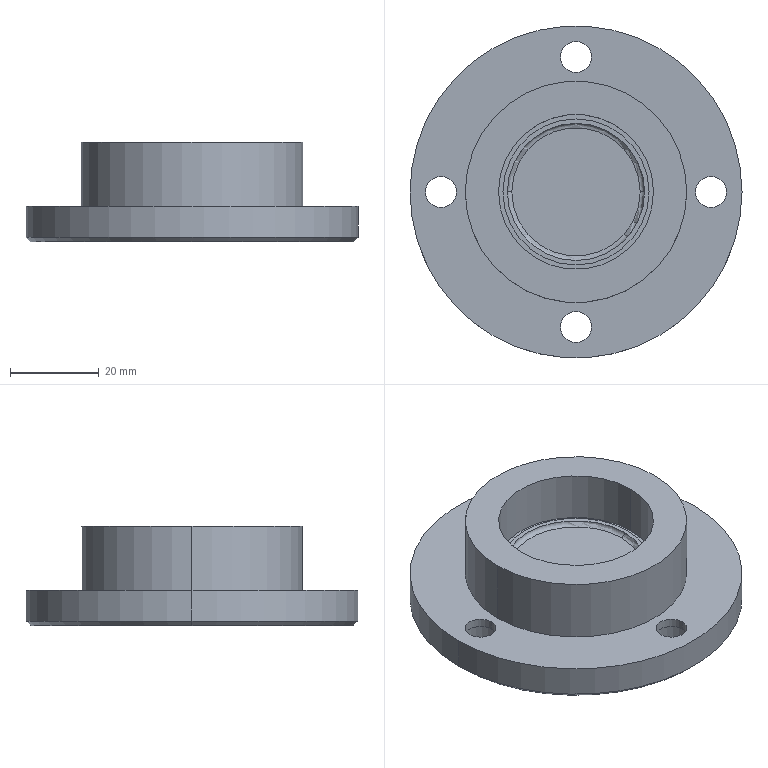Part | SolidWorks | features ICE 7, Chamfer 1, CirPattern 1, Extrusion 1, Fillet 1 | 1 solid | 41 faces | box 75 x 75 x 22.5 mm | volume 47960 mm3 | cylinder 24 | plane 11 | torus 4 | cone 2 | commonest cylinder face diameters 7 x8 11 x8 33 x2 35 x2 50 x2 75 x2
STEP:
#1=CARTESIAN_POINT('',(-36.5,0.,0.));
#2=VERTEX_POINT('',#1);
#3=CARTESIAN_POINT('',(36.5,0.,0.));
#4=VERTEX_POINT('',#3);
#5=CARTESIAN_POINT('',(0.,0.,0.));
#6=DIRECTION('',(0.,0.,-1.));
#7=DIRECTION('',(1.,0.,0.));
#8=AXIS2_PLACEMENT_3D('',#5,#6,#7);
#9=CIRCLE('',#8,36.5);
#10=EDGE_CURVE('',#2,#4,#9,.T.);
#11=ORIENTED_EDGE('',*,*,#10,.F.);
#12=CARTESIAN_POINT('',(-37.5,0.,1.));
#13=VERTEX_POINT('',#12);
#14=CARTESIAN_POINT('',(-37.5,0.,1.));
#15=DIRECTION('',(-0.7071,0.,0.7071));
#16=VECTOR('',#15,1000.);
#17=LINE('',#14,#16);
#18=EDGE_CURVE('',#2,#13,#17,.T.);
#19=ORIENTED_EDGE('',*,*,#18,.T.);
#20=CARTESIAN_POINT('',(37.5,0.,1.));
#21=VERTEX_POINT('',#20);
#22=CARTESIAN_POINT('',(0.,0.,1.));
#23=DIRECTION('',(0.,0.,1.));
#24=DIRECTION('',(1.,0.,0.));
#25=AXIS2_PLACEMENT_3D('',#22,#23,#24);
#26=CIRCLE('',#25,37.5);
#27=EDGE_CURVE('',#21,#13,#26,.T.);
#28=ORIENTED_EDGE('',*,*,#27,.F.);
#29=CARTESIAN_POINT('',(37.5,0.,1.));
#30=DIRECTION('',(0.7071,0.,0.7071));
#31=VECTOR('',#30,1000.);
#32=LINE('',#29,#31);
#33=EDGE_CURVE('',#4,#21,#32,.T.);
#34=ORIENTED_EDGE('',*,*,#33,.F.);
#35=EDGE_LOOP('',(#11,#19,#28,#34));
#36=FACE_OUTER_BOUND('',#35,.T.);
#37=CARTESIAN_POINT('',(0.,0.,1.));
#38=DIRECTION('',(0.,0.,1.));
#39=DIRECTION('',(1.,0.,0.));
#40=AXIS2_PLACEMENT_3D('',#37,#38,#39);
#41=CONICAL_SURFACE('',#40,37.5,0.7854);
#42=ADVANCED_FACE('',(#36),#41,.T.);
#43=CARTESIAN_POINT('',(-14.5,0.,10.5));
#44=VERTEX_POINT('',#43);
#45=CARTESIAN_POINT('',(14.5,0.,10.5));
#46=VERTEX_POINT('',#45);
#47=CARTESIAN_POINT('',(0.,0.,10.5));
#48=DIRECTION('',(0.,0.,1.));
#49=DIRECTION('',(1.,0.,0.));
#50=AXIS2_PLACEMENT_3D('',#47,#48,#49);
#51=CIRCLE('',#50,14.5);
#52=EDGE_CURVE('',#44,#46,#51,.T.);
#53=ORIENTED_EDGE('',*,*,#52,.F.);
#54=CARTESIAN_POINT('',(-15.5,0.,11.5));
#55=VERTEX_POINT('',#54);
#56=CARTESIAN_POINT('',(-14.5,0.,11.5));
#57=DIRECTION('',(0.,1.,0.));
#58=DIRECTION('',(-1.,0.,0.));
#59=AXIS2_PLACEMENT_3D('',#56,#57,#58);
#60=CIRCLE('',#59,1.);
#61=EDGE_CURVE('',#44,#55,#60,.T.);
#62=ORIENTED_EDGE('',*,*,#61,.T.);
#63=CARTESIAN_POINT('',(15.5,0.,11.5));
#64=VERTEX_POINT('',#63);
#65=CARTESIAN_POINT('',(0.,0.,11.5));
#66=DIRECTION('',(0.,0.,1.));
#67=DIRECTION('',(1.,0.,0.));
#68=AXIS2_PLACEMENT_3D('',#65,#66,#67);
#69=CIRCLE('',#68,15.5);
#70=EDGE_CURVE('',#55,#64,#69,.T.);
#71=ORIENTED_EDGE('',*,*,#70,.T.);
#72=CARTESIAN_POINT('',(14.5,0.,11.5));
#73=DIRECTION('',(0.,-1.,0.));
#74=DIRECTION('',(0.,0.,-1.));
#75=AXIS2_PLACEMENT_3D('',#72,#73,#74);
#76=CIRCLE('',#75,1.);
#77=EDGE_CURVE('',#46,#64,#76,.T.);
#78=ORIENTED_EDGE('',*,*,#77,.F.);
#79=EDGE_LOOP('',(#53,#62,#71,#78));
#80=FACE_OUTER_BOUND('',#79,.T.);
#81=CARTESIAN_POINT('',(0.,0.,11.5));
#82=DIRECTION('',(0.,0.,1.));
#83=DIRECTION('',(1.,0.,0.));
#84=AXIS2_PLACEMENT_3D('',#81,#82,#83);
#85=TOROIDAL_SURFACE('',#84,14.5,1.);
#86=ADVANCED_FACE('',(#80),#85,.F.);
#87=CARTESIAN_POINT('',(23.,0.,1.));
#88=VERTEX_POINT('',#87);
#89=CARTESIAN_POINT('',(-23.,0.,1.));
#90=VERTEX_POINT('',#89);
#91=CARTESIAN_POINT('',(0.,0.,1.));
#92=DIRECTION('',(0.,0.,-1.));
#93=DIRECTION('',(-1.,0.,0.));
#94=AXIS2_PLACEMENT_3D('',#91,#92,#93);
#95=CIRCLE('',#94,23.);
#96=EDGE_CURVE('',#88,#90,#95,.T.);
#97=ORIENTED_EDGE('',*,*,#96,.F.);
#98=CARTESIAN_POINT('',(24.,0.,0.));
#99=VERTEX_POINT('',#98);
#100=CARTESIAN_POINT('',(23.,0.,0.));
#101=DIRECTION('',(0.,1.,0.));
#102=DIRECTION('',(-1.,0.,0.));
#103=AXIS2_PLACEMENT_3D('',#100,#101,#102);
#104=CIRCLE('',#103,1.);
#105=EDGE_CURVE('',#88,#99,#104,.T.);
#106=ORIENTED_EDGE('',*,*,#105,.T.);
#107=CARTESIAN_POINT('',(-24.,0.,0.));
#108=VERTEX_POINT('',#107);
#109=CARTESIAN_POINT('',(0.,0.,0.));
#110=DIRECTION('',(0.,0.,-1.));
#111=DIRECTION('',(-1.,0.,0.));
#112=AXIS2_PLACEMENT_3D('',#109,#110,#111);
#113=CIRCLE('',#112,24.);
#114=EDGE_CURVE('',#99,#108,#113,.T.);
#115=ORIENTED_EDGE('',*,*,#114,.T.);
#116=CARTESIAN_POINT('',(-23.,0.,0.));
#117=DIRECTION('',(0.,-1.,0.));
#118=DIRECTION('',(0.,0.,-1.));
#119=AXIS2_PLACEMENT_3D('',#116,#117,#118);
#120=CIRCLE('',#119,1.);
#121=EDGE_CURVE('',#90,#108,#120,.T.);
#122=ORIENTED_EDGE('',*,*,#121,.F.);
#123=EDGE_LOOP('',(#97,#106,#115,#122));
#124=FACE_OUTER_BOUND('',#123,.T.);
#125=CARTESIAN_POINT('',(0.,0.,0.));
#126=DIRECTION('',(0.,0.,-1.));
#127=DIRECTION('',(-1.,0.,0.));
#128=AXIS2_PLACEMENT_3D('',#125,#126,#127);
#129=TOROIDAL_SURFACE('',#128,23.,1.);
#130=ADVANCED_FACE('',(#124),#129,.F.);
#131=CARTESIAN_POINT('',(16.5,0.,11.));
#132=VERTEX_POINT('',#131);
#133=CARTESIAN_POINT('',(-16.5,0.,11.));
#134=VERTEX_POINT('',#133);
#135=CARTESIAN_POINT('',(0.,0.,11.));
#136=DIRECTION('',(0.,0.,1.));
#137=DIRECTION('',(1.,0.,0.));
#138=AXIS2_PLACEMENT_3D('',#135,#136,#137);
#139=CIRCLE('',#138,16.5);
#140=EDGE_CURVE('',#132,#134,#139,.T.);
#141=ORIENTED_EDGE('',*,*,#140,.T.);
#142=CARTESIAN_POINT('',(-16.5,0.,11.5));
#143=VERTEX_POINT('',#142);
#144=CARTESIAN_POINT('',(-16.5,0.,11.));
#145=DIRECTION('',(0.,0.,1.));
#146=VECTOR('',#145,1000.);
#147=LINE('',#144,#146);
#148=EDGE_CURVE('',#134,#143,#147,.T.);
#149=ORIENTED_EDGE('',*,*,#148,.T.);
#150=CARTESIAN_POINT('',(16.5,0.,11.5));
#151=VERTEX_POINT('',#150);
#152=CARTESIAN_POINT('',(0.,0.,11.5));
#153=DIRECTION('',(0.,0.,1.));
#154=DIRECTION('',(1.,0.,0.));
#155=AXIS2_PLACEMENT_3D('',#152,#153,#154);
#156=CIRCLE('',#155,16.5);
#157=EDGE_CURVE('',#151,#143,#156,.T.);
#158=ORIENTED_EDGE('',*,*,#157,.F.);
#159=CARTESIAN_POINT('',(16.5,0.,11.));
#160=DIRECTION('',(0.,0.,1.));
#161=VECTOR('',#160,1000.);
#162=LINE('',#159,#161);
#163=EDGE_CURVE('',#132,#151,#162,.T.);
#164=ORIENTED_EDGE('',*,*,#163,.F.);
#165=EDGE_LOOP('',(#141,#149,#158,#164));
#166=FACE_OUTER_BOUND('',#165,.T.);
#167=CARTESIAN_POINT('',(0.,0.,11.));
#168=DIRECTION('',(0.,0.,1.));
#169=DIRECTION('',(1.,0.,0.));
#170=AXIS2_PLACEMENT_3D('',#167,#168,#169);
#171=CYLINDRICAL_SURFACE('',#170,16.5);
#172=ADVANCED_FACE('',(#166),#171,.T.);
#173=CARTESIAN_POINT('',(-17.5,0.,11.));
#174=VERTEX_POINT('',#173);
#175=CARTESIAN_POINT('',(17.5,0.,11.));
#176=VERTEX_POINT('',#175);
#177=CARTESIAN_POINT('',(0.,0.,11.));
#178=DIRECTION('',(0.,0.,1.));
#179=DIRECTION('',(1.,0.,0.));
#180=AXIS2_PLACEMENT_3D('',#177,#178,#179);
#181=CIRCLE('',#180,17.5);
#182=EDGE_CURVE('',#174,#176,#181,.T.);
#183=ORIENTED_EDGE('',*,*,#182,.F.);
#184=CARTESIAN_POINT('',(-17.5,0.,22.5));
#185=VERTEX_POINT('',#184);
#186=CARTESIAN_POINT('',(-17.5,0.,11.5));
#187=DIRECTION('',(0.,0.,1.));
#188=VECTOR('',#187,1000.);
#189=LINE('',#186,#188);
#190=EDGE_CURVE('',#174,#185,#189,.T.);
#191=ORIENTED_EDGE('',*,*,#190,.T.);
#192=CARTESIAN_POINT('',(17.5,0.,22.5));
#193=VERTEX_POINT('',#192);
#194=CARTESIAN_POINT('',(0.,0.,22.5));
#195=DIRECTION('',(0.,0.,1.));
#196=DIRECTION('',(1.,0.,0.));
#197=AXIS2_PLACEMENT_3D('',#194,#195,#196);
#198=CIRCLE('',#197,17.5);
#199=EDGE_CURVE('',#185,#193,#198,.T.);
#200=ORIENTED_EDGE('',*,*,#199,.T.);
#201=CARTESIAN_POINT('',(17.5,0.,11.5));
#202=DIRECTION('',(0.,0.,1.));
#203=VECTOR('',#202,1000.);
#204=LINE('',#201,#203);
#205=EDGE_CURVE('',#176,#193,#204,.T.);
#206=ORIENTED_EDGE('',*,*,#205,.F.);
#207=EDGE_LOOP('',(#183,#191,#200,#206));
#208=FACE_OUTER_BOUND('',#207,.T.);
#209=CARTESIAN_POINT('',(0.,0.,11.5));
#210=DIRECTION('',(0.,0.,1.));
#211=DIRECTION('',(1.,0.,0.));
#212=AXIS2_PLACEMENT_3D('',#209,#210,#211);
#213=CYLINDRICAL_SURFACE('',#212,17.5);
#214=ADVANCED_FACE('',(#208),#213,.F.);
#215=CARTESIAN_POINT('',(27.,0.,8.));
#216=VERTEX_POINT('',#215);
#217=CARTESIAN_POINT('',(34.,0.,8.));
#218=VERTEX_POINT('',#217);
#219=CARTESIAN_POINT('',(30.5,0.,8.));
#220=DIRECTION('',(0.,0.,1.));
#221=DIRECTION('',(1.,0.,0.));
#222=AXIS2_PLACEMENT_3D('',#219,#220,#221);
#223=CIRCLE('',#222,3.5);
#224=EDGE_CURVE('',#216,#218,#223,.T.);
#225=ORIENTED_EDGE('',*,*,#224,.T.);
#226=CARTESIAN_POINT('',(34.,0.,6.));
#227=VERTEX_POINT('',#226);
#228=CARTESIAN_POINT('',(34.,0.,27.));
#229=DIRECTION('',(0.,0.,-1.));
#230=VECTOR('',#229,1000.);
#231=LINE('',#228,#230);
#232=EDGE_CURVE('',#218,#227,#231,.T.);
#233=ORIENTED_EDGE('',*,*,#232,.T.);
#234=CARTESIAN_POINT('',(27.,0.,6.));
#235=VERTEX_POINT('',#234);
#236=CARTESIAN_POINT('',(30.5,0.,6.));
#237=DIRECTION('',(0.,0.,-1.));
#238=DIRECTION('',(0.,1.,0.));
#239=AXIS2_PLACEMENT_3D('',#236,#237,#238);
#240=CIRCLE('',#239,3.5);
#241=EDGE_CURVE('',#227,#235,#240,.T.);
#242=ORIENTED_EDGE('',*,*,#241,.T.);
#243=CARTESIAN_POINT('',(27.,0.,27.));
#244=DIRECTION('',(0.,0.,-1.));
#245=VECTOR('',#244,1000.);
#246=LINE('',#243,#245);
#247=EDGE_CURVE('',#216,#235,#246,.T.);
#248=ORIENTED_EDGE('',*,*,#247,.F.);
#249=EDGE_LOOP('',(#225,#233,#242,#248));
#250=FACE_OUTER_BOUND('',#249,.T.);
#251=CARTESIAN_POINT('',(30.5,0.,27.));
#252=DIRECTION('',(0.,0.,-1.));
#253=DIRECTION('',(-1.,0.,0.));
#254=AXIS2_PLACEMENT_3D('',#251,#252,#253);
#255=CYLINDRICAL_SURFACE('',#254,3.5);
#256=ADVANCED_FACE('',(#250),#255,.F.);
#257=CARTESIAN_POINT('',(-3.5,-30.5,8.));
#258=VERTEX_POINT('',#257);
#259=CARTESIAN_POINT('',(3.5,-30.5,8.));
#260=VERTEX_POINT('',#259);
#261=CARTESIAN_POINT('',(0.,-30.5,8.));
#262=DIRECTION('',(0.,0.,1.));
#263=DIRECTION('',(1.,0.,0.));
#264=AXIS2_PLACEMENT_3D('',#261,#262,#263);
#265=CIRCLE('',#264,3.5);
#266=EDGE_CURVE('',#258,#260,#265,.T.);
#267=ORIENTED_EDGE('',*,*,#266,.T.);
#268=CARTESIAN_POINT('',(3.5,-30.5,6.));
#269=VERTEX_POINT('',#268);
#270=CARTESIAN_POINT('',(3.5,-30.5,27.));
#271=DIRECTION('',(0.,0.,-1.));
#272=VECTOR('',#271,1000.);
#273=LINE('',#270,#272);
#274=EDGE_CURVE('',#260,#269,#273,.T.);
#275=ORIENTED_EDGE('',*,*,#274,.T.);
#276=CARTESIAN_POINT('',(-3.5,-30.5,6.));
#277=VERTEX_POINT('',#276);
#278=CARTESIAN_POINT('',(0.,-30.5,6.));
#279=DIRECTION('',(0.,0.,-1.));
#280=DIRECTION('',(1.,0.,0.));
#281=AXIS2_PLACEMENT_3D('',#278,#279,#280);
#282=CIRCLE('',#281,3.5);
#283=EDGE_CURVE('',#269,#277,#282,.T.);
#284=ORIENTED_EDGE('',*,*,#283,.T.);
#285=CARTESIAN_POINT('',(-3.5,-30.5,27.));
#286=DIRECTION('',(0.,0.,-1.));
#287=VECTOR('',#286,1000.);
#288=LINE('',#285,#287);
#289=EDGE_CURVE('',#258,#277,#288,.T.);
#290=ORIENTED_EDGE('',*,*,#289,.F.);
#291=EDGE_LOOP('',(#267,#275,#284,#290));
#292=FACE_OUTER_BOUND('',#291,.T.);
#293=CARTESIAN_POINT('',(0.,-30.5,27.));
#294=DIRECTION('',(0.,0.,-1.));
#295=DIRECTION('',(-1.,0.,0.));
#296=AXIS2_PLACEMENT_3D('',#293,#294,#295);
#297=CYLINDRICAL_SURFACE('',#296,3.5);
#298=ADVANCED_FACE('',(#292),#297,.F.);
#299=CARTESIAN_POINT('',(-34.,0.,8.));
#300=VERTEX_POINT('',#299);
#301=CARTESIAN_POINT('',(-27.,0.,8.));
#302=VERTEX_POINT('',#301);
#303=CARTESIAN_POINT('',(-30.5,0.,8.));
#304=DIRECTION('',(0.,0.,1.));
#305=DIRECTION('',(1.,0.,0.));
#306=AXIS2_PLACEMENT_3D('',#303,#304,#305);
#307=CIRCLE('',#306,3.5);
#308=EDGE_CURVE('',#300,#302,#307,.T.);
#309=ORIENTED_EDGE('',*,*,#308,.T.);
#310=CARTESIAN_POINT('',(-27.,0.,6.));
#311=VERTEX_POINT('',#310);
#312=CARTESIAN_POINT('',(-27.,0.,27.));
#313=DIRECTION('',(0.,0.,-1.));
#314=VECTOR('',#313,1000.);
#315=LINE('',#312,#314);
#316=EDGE_CURVE('',#302,#311,#315,.T.);
#317=ORIENTED_EDGE('',*,*,#316,.T.);
#318=CARTESIAN_POINT('',(-34.,0.,6.));
#319=VERTEX_POINT('',#318);
#320=CARTESIAN_POINT('',(-30.5,0.,6.));
#321=DIRECTION('',(0.,0.,-1.));
#322=DIRECTION('',(0.,-1.,0.));
#323=AXIS2_PLACEMENT_3D('',#320,#321,#322);
#324=CIRCLE('',#323,3.5);
#325=EDGE_CURVE('',#311,#319,#324,.T.);
#326=ORIENTED_EDGE('',*,*,#325,.T.);
#327=CARTESIAN_POINT('',(-34.,0.,27.));
#328=DIRECTION('',(0.,0.,-1.));
#329=VECTOR('',#328,1000.);
#330=LINE('',#327,#329);
#331=EDGE_CURVE('',#300,#319,#330,.T.);
#332=ORIENTED_EDGE('',*,*,#331,.F.);
#333=EDGE_LOOP('',(#309,#317,#326,#332));
#334=FACE_OUTER_BOUND('',#333,.T.);
#335=CARTESIAN_POINT('',(-30.5,0.,27.));
#336=DIRECTION('',(0.,0.,-1.));
#337=DIRECTION('',(-1.,0.,0.));
#338=AXIS2_PLACEMENT_3D('',#335,#336,#337);
#339=CYLINDRICAL_SURFACE('',#338,3.5);
#340=ADVANCED_FACE('',(#334),#339,.F.);
#341=CARTESIAN_POINT('',(36.,0.,6.));
#342=VERTEX_POINT('',#341);
#343=CARTESIAN_POINT('',(25.,0.,6.));
#344=VERTEX_POINT('',#343);
#345=CARTESIAN_POINT('',(30.5,0.,6.));
#346=DIRECTION('',(0.,0.,-1.));
#347=DIRECTION('',(0.,1.,0.));
#348=AXIS2_PLACEMENT_3D('',#345,#346,#347);
#349=CIRCLE('',#348,5.5);
#350=EDGE_CURVE('',#342,#344,#349,.T.);
#351=ORIENTED_EDGE('',*,*,#350,.F.);
#352=CARTESIAN_POINT('',(36.,0.,0.));
#353=VERTEX_POINT('',#352);
#354=CARTESIAN_POINT('',(36.,0.,6.));
#355=DIRECTION('',(0.,0.,-1.));
#356=VECTOR('',#355,1000.);
#357=LINE('',#354,#356);
#358=EDGE_CURVE('',#342,#353,#357,.T.);
#359=ORIENTED_EDGE('',*,*,#358,.T.);
#360=CARTESIAN_POINT('',(25.,0.,0.));
#361=VERTEX_POINT('',#360);
#362=CARTESIAN_POINT('',(30.5,0.,0.));
#363=DIRECTION('',(0.,0.,-1.));
#364=DIRECTION('',(0.,1.,0.));
#365=AXIS2_PLACEMENT_3D('',#362,#363,#364);
#366=CIRCLE('',#365,5.5);
#367=EDGE_CURVE('',#353,#361,#366,.T.);
#368=ORIENTED_EDGE('',*,*,#367,.T.);
#369=CARTESIAN_POINT('',(25.,0.,6.));
#370=DIRECTION('',(0.,0.,-1.));
#371=VECTOR('',#370,1000.);
#372=LINE('',#369,#371);
#373=EDGE_CURVE('',#344,#361,#372,.T.);
#374=ORIENTED_EDGE('',*,*,#373,.F.);
#375=EDGE_LOOP('',(#351,#359,#368,#374));
#376=FACE_OUTER_BOUND('',#375,.T.);
#377=CARTESIAN_POINT('',(30.5,0.,6.));
#378=DIRECTION('',(0.,0.,-1.));
#379=DIRECTION('',(-1.,0.,0.));
#380=AXIS2_PLACEMENT_3D('',#377,#378,#379);
#381=CYLINDRICAL_SURFACE('',#380,5.5);
#382=ADVANCED_FACE('',(#376),#381,.F.);
#383=CARTESIAN_POINT('',(5.5,-30.5,6.));
#384=VERTEX_POINT('',#383);
#385=CARTESIAN_POINT('',(-5.5,-30.5,6.));
#386=VERTEX_POINT('',#385);
#387=CARTESIAN_POINT('',(0.,-30.5,6.));
#388=DIRECTION('',(0.,0.,-1.));
#389=DIRECTION('',(1.,0.,0.));
#390=AXIS2_PLACEMENT_3D('',#387,#388,#389);
#391=CIRCLE('',#390,5.5);
#392=EDGE_CURVE('',#384,#386,#391,.T.);
#393=ORIENTED_EDGE('',*,*,#392,.F.);
#394=CARTESIAN_POINT('',(5.5,-30.5,0.));
#395=VERTEX_POINT('',#394);
#396=CARTESIAN_POINT('',(5.5,-30.5,6.));
#397=DIRECTION('',(0.,0.,-1.));
#398=VECTOR('',#397,1000.);
#399=LINE('',#396,#398);
#400=EDGE_CURVE('',#384,#395,#399,.T.);
#401=ORIENTED_EDGE('',*,*,#400,.T.);
#402=CARTESIAN_POINT('',(-5.5,-30.5,0.));
#403=VERTEX_POINT('',#402);
#404=CARTESIAN_POINT('',(0.,-30.5,0.));
#405=DIRECTION('',(0.,0.,-1.));
#406=DIRECTION('',(1.,0.,0.));
#407=AXIS2_PLACEMENT_3D('',#404,#405,#406);
#408=CIRCLE('',#407,5.5);
#409=EDGE_CURVE('',#395,#403,#408,.T.);
#410=ORIENTED_EDGE('',*,*,#409,.T.);
#411=CARTESIAN_POINT('',(-5.5,-30.5,6.));
#412=DIRECTION('',(0.,0.,-1.));
#413=VECTOR('',#412,1000.);
#414=LINE('',#411,#413);
#415=EDGE_CURVE('',#386,#403,#414,.T.);
#416=ORIENTED_EDGE('',*,*,#415,.F.);
#417=EDGE_LOOP('',(#393,#401,#410,#416));
#418=FACE_OUTER_BOUND('',#417,.T.);
#419=CARTESIAN_POINT('',(0.,-30.5,6.));
#420=DIRECTION('',(0.,0.,-1.));
#421=DIRECTION('',(-1.,0.,0.));
#422=AXIS2_PLACEMENT_3D('',#419,#420,#421);
#423=CYLINDRICAL_SURFACE('',#422,5.5);
#424=ADVANCED_FACE('',(#418),#423,.F.);
#425=CARTESIAN_POINT('',(-25.,0.,6.));
#426=VERTEX_POINT('',#425);
#427=CARTESIAN_POINT('',(-36.,0.,6.));
#428=VERTEX_POINT('',#427);
#429=CARTESIAN_POINT('',(-30.5,0.,6.));
#430=DIRECTION('',(0.,0.,-1.));
#431=DIRECTION('',(0.,-1.,0.));
#432=AXIS2_PLACEMENT_3D('',#429,#430,#431);
#433=CIRCLE('',#432,5.5);
#434=EDGE_CURVE('',#426,#428,#433,.T.);
#435=ORIENTED_EDGE('',*,*,#434,.F.);
#436=CARTESIAN_POINT('',(-25.,0.,0.));
#437=VERTEX_POINT('',#436);
#438=CARTESIAN_POINT('',(-25.,0.,6.));
#439=DIRECTION('',(0.,0.,-1.));
#440=VECTOR('',#439,1000.);
#441=LINE('',#438,#440);
#442=EDGE_CURVE('',#426,#437,#441,.T.);
#443=ORIENTED_EDGE('',*,*,#442,.T.);
#444=CARTESIAN_POINT('',(-36.,0.,0.));
#445=VERTEX_POINT('',#444);
#446=CARTESIAN_POINT('',(-30.5,0.,0.));
#447=DIRECTION('',(0.,0.,-1.));
#448=DIRECTION('',(0.,-1.,0.));
#449=AXIS2_PLACEMENT_3D('',#446,#447,#448);
#450=CIRCLE('',#449,5.5);
#451=EDGE_CURVE('',#437,#445,#450,.T.);
#452=ORIENTED_EDGE('',*,*,#451,.T.);
#453=CARTESIAN_POINT('',(-36.,0.,6.));
#454=DIRECTION('',(0.,0.,-1.));
#455=VECTOR('',#454,1000.);
#456=LINE('',#453,#455);
#457=EDGE_CURVE('',#428,#445,#456,.T.);
#458=ORIENTED_EDGE('',*,*,#457,.F.);
#459=EDGE_LOOP('',(#435,#443,#452,#458));
#460=FACE_OUTER_BOUND('',#459,.T.);
#461=CARTESIAN_POINT('',(-30.5,0.,6.));
#462=DIRECTION('',(0.,0.,-1.));
#463=DIRECTION('',(-1.,0.,0.));
#464=AXIS2_PLACEMENT_3D('',#461,#462,#463);
#465=CYLINDRICAL_SURFACE('',#464,5.5);
#466=ADVANCED_FACE('',(#460),#465,.F.);
#467=CARTESIAN_POINT('',(-3.5,30.5,8.));
#468=VERTEX_POINT('',#467);
#469=CARTESIAN_POINT('',(3.5,30.5,8.));
#470=VERTEX_POINT('',#469);
#471=CARTESIAN_POINT('',(0.,30.5,8.));
#472=DIRECTION('',(0.,0.,1.));
#473=DIRECTION('',(1.,0.,0.));
#474=AXIS2_PLACEMENT_3D('',#471,#472,#473);
#475=CIRCLE('',#474,3.5);
#476=EDGE_CURVE('',#468,#470,#475,.T.);
#477=ORIENTED_EDGE('',*,*,#476,.T.);
#478=CARTESIAN_POINT('',(3.5,30.5,6.));
#479=VERTEX_POINT('',#478);
#480=CARTESIAN_POINT('',(3.5,30.5,27.));
#481=DIRECTION('',(0.,0.,-1.));
#482=VECTOR('',#481,1000.);
#483=LINE('',#480,#482);
#484=EDGE_CURVE('',#470,#479,#483,.T.);
#485=ORIENTED_EDGE('',*,*,#484,.T.);
#486=CARTESIAN_POINT('',(-3.5,30.5,6.));
#487=VERTEX_POINT('',#486);
#488=CARTESIAN_POINT('',(0.,30.5,6.));
#489=DIRECTION('',(0.,0.,-1.));
#490=DIRECTION('',(-1.,0.,0.));
#491=AXIS2_PLACEMENT_3D('',#488,#489,#490);
#492=CIRCLE('',#491,3.5);
#493=EDGE_CURVE('',#479,#487,#492,.T.);
#494=ORIENTED_EDGE('',*,*,#493,.T.);
#495=CARTESIAN_POINT('',(-3.5,30.5,27.));
#496=DIRECTION('',(0.,0.,-1.));
#497=VECTOR('',#496,1000.);
#498=LINE('',#495,#497);
#499=EDGE_CURVE('',#468,#487,#498,.T.);
#500=ORIENTED_EDGE('',*,*,#499,.F.);
#501=EDGE_LOOP('',(#477,#485,#494,#500));
#502=FACE_OUTER_BOUND('',#501,.T.);
#503=CARTESIAN_POINT('',(0.,30.5,27.));
#504=DIRECTION('',(0.,0.,-1.));
#505=DIRECTION('',(-1.,0.,0.));
#506=AXIS2_PLACEMENT_3D('',#503,#504,#505);
#507=CYLINDRICAL_SURFACE('',#506,3.5);
#508=ADVANCED_FACE('',(#502),#507,.F.);
#509=CARTESIAN_POINT('',(5.5,30.5,6.));
#510=VERTEX_POINT('',#509);
#511=CARTESIAN_POINT('',(-5.5,30.5,6.));
#512=VERTEX_POINT('',#511);
#513=CARTESIAN_POINT('',(0.,30.5,6.));
#514=DIRECTION('',(0.,0.,-1.));
#515=DIRECTION('',(-1.,0.,0.));
#516=AXIS2_PLACEMENT_3D('',#513,#514,#515);
#517=CIRCLE('',#516,5.5);
#518=EDGE_CURVE('',#510,#512,#517,.T.);
#519=ORIENTED_EDGE('',*,*,#518,.F.);
#520=CARTESIAN_POINT('',(5.5,30.5,0.));
#521=VERTEX_POINT('',#520);
#522=CARTESIAN_POINT('',(5.5,30.5,6.));
#523=DIRECTION('',(0.,0.,-1.));
#524=VECTOR('',#523,1000.);
#525=LINE('',#522,#524);
#526=EDGE_CURVE('',#510,#521,#525,.T.);
#527=ORIENTED_EDGE('',*,*,#526,.T.);
#528=CARTESIAN_POINT('',(-5.5,30.5,0.));
#529=VERTEX_POINT('',#528);
#530=CARTESIAN_POINT('',(0.,30.5,0.));
#531=DIRECTION('',(0.,0.,-1.));
#532=DIRECTION('',(-1.,0.,0.));
#533=AXIS2_PLACEMENT_3D('',#530,#531,#532);
#534=CIRCLE('',#533,5.5);
#535=EDGE_CURVE('',#521,#529,#534,.T.);
#536=ORIENTED_EDGE('',*,*,#535,.T.);
#537=CARTESIAN_POINT('',(-5.5,30.5,6.));
#538=DIRECTION('',(0.,0.,-1.));
#539=VECTOR('',#538,1000.);
#540=LINE('',#537,#539);
#541=EDGE_CURVE('',#512,#529,#540,.T.);
#542=ORIENTED_EDGE('',*,*,#541,.F.);
#543=EDGE_LOOP('',(#519,#527,#536,#542));
#544=FACE_OUTER_BOUND('',#543,.T.);
#545=CARTESIAN_POINT('',(0.,30.5,6.));
#546=DIRECTION('',(0.,0.,-1.));
#547=DIRECTION('',(-1.,0.,0.));
#548=AXIS2_PLACEMENT_3D('',#545,#546,#547);
#549=CYLINDRICAL_SURFACE('',#548,5.5);
#550=ADVANCED_FACE('',(#544),#549,.F.);
#551=CARTESIAN_POINT('',(25.,0.,22.5));
#552=VERTEX_POINT('',#551);
#553=CARTESIAN_POINT('',(-25.,0.,22.5));
#554=VERTEX_POINT('',#553);
#555=CARTESIAN_POINT('',(0.,0.,22.5));
#556=DIRECTION('',(0.,0.,1.));
#557=DIRECTION('',(1.,0.,0.));
#558=AXIS2_PLACEMENT_3D('',#555,#556,#557);
#559=CIRCLE('',#558,25.);
#560=EDGE_CURVE('',#552,#554,#559,.T.);
#561=ORIENTED_EDGE('',*,*,#560,.F.);
#562=CARTESIAN_POINT('',(25.,0.,8.));
#563=VERTEX_POINT('',#562);
#564=CARTESIAN_POINT('',(25.,0.,22.5));
#565=DIRECTION('',(0.,0.,-1.));
#566=VECTOR('',#565,1000.);
#567=LINE('',#564,#566);
#568=EDGE_CURVE('',#552,#563,#567,.T.);
#569=ORIENTED_EDGE('',*,*,#568,.T.);
#570=CARTESIAN_POINT('',(-25.,0.,8.));
#571=VERTEX_POINT('',#570);
#572=CARTESIAN_POINT('',(0.,0.,8.));
#573=DIRECTION('',(0.,0.,1.));
#574=DIRECTION('',(1.,0.,0.));
#575=AXIS2_PLACEMENT_3D('',#572,#573,#574);
#576=CIRCLE('',#575,25.);
#577=EDGE_CURVE('',#563,#571,#576,.T.);
#578=ORIENTED_EDGE('',*,*,#577,.T.);
#579=CARTESIAN_POINT('',(-25.,0.,22.5));
#580=DIRECTION('',(0.,0.,-1.));
#581=VECTOR('',#580,1000.);
#582=LINE('',#579,#581);
#583=EDGE_CURVE('',#554,#571,#582,.T.);
#584=ORIENTED_EDGE('',*,*,#583,.F.);
#585=EDGE_LOOP('',(#561,#569,#578,#584));
#586=FACE_OUTER_BOUND('',#585,.T.);
#587=CARTESIAN_POINT('',(0.,0.,22.5));
#588=DIRECTION('',(0.,0.,-1.));
#589=DIRECTION('',(-1.,0.,0.));
#590=AXIS2_PLACEMENT_3D('',#587,#588,#589);
#591=CYLINDRICAL_SURFACE('',#590,25.);
#592=ADVANCED_FACE('',(#586),#591,.T.);
#593=CARTESIAN_POINT('',(37.5,0.,8.));
#594=VERTEX_POINT('',#593);
#595=CARTESIAN_POINT('',(-37.5,0.,8.));
#596=VERTEX_POINT('',#595);
#597=CARTESIAN_POINT('',(0.,0.,8.));
#598=DIRECTION('',(0.,0.,1.));
#599=DIRECTION('',(1.,0.,0.));
#600=AXIS2_PLACEMENT_3D('',#597,#598,#599);
#601=CIRCLE('',#600,37.5);
#602=EDGE_CURVE('',#594,#596,#601,.T.);
#603=ORIENTED_EDGE('',*,*,#602,.F.);
#604=CARTESIAN_POINT('',(37.5,0.,8.));
#605=DIRECTION('',(0.,0.,-1.));
#606=VECTOR('',#605,1000.);
#607=LINE('',#604,#606);
#608=EDGE_CURVE('',#594,#21,#607,.T.);
#609=ORIENTED_EDGE('',*,*,#608,.T.);
#610=ORIENTED_EDGE('',*,*,#27,.T.);
#611=CARTESIAN_POINT('',(-37.5,0.,8.));
#612=DIRECTION('',(0.,0.,-1.));
#613=VECTOR('',#612,1000.);
#614=LINE('',#611,#613);
#615=EDGE_CURVE('',#596,#13,#614,.T.);
#616=ORIENTED_EDGE('',*,*,#615,.F.);
#617=EDGE_LOOP('',(#603,#609,#610,#616));
#618=FACE_OUTER_BOUND('',#617,.T.);
#619=CARTESIAN_POINT('',(0.,0.,8.));
#620=DIRECTION('',(0.,0.,-1.));
#621=DIRECTION('',(-1.,0.,0.));
#622=AXIS2_PLACEMENT_3D('',#619,#620,#621);
#623=CYLINDRICAL_SURFACE('',#622,37.5);
#624=ADVANCED_FACE('',(#618),#623,.T.);
#625=ORIENTED_EDGE('',*,*,#608,.F.);
#626=CARTESIAN_POINT('',(0.,0.,8.));
#627=DIRECTION('',(0.,0.,1.));
#628=DIRECTION('',(1.,0.,0.));
#629=AXIS2_PLACEMENT_3D('',#626,#627,#628);
#630=CIRCLE('',#629,37.5);
#631=EDGE_CURVE('',#596,#594,#630,.T.);
#632=ORIENTED_EDGE('',*,*,#631,.F.);
#633=ORIENTED_EDGE('',*,*,#615,.T.);
#634=CARTESIAN_POINT('',(0.,0.,1.));
#635=DIRECTION('',(0.,0.,1.));
#636=DIRECTION('',(1.,0.,0.));
#637=AXIS2_PLACEMENT_3D('',#634,#635,#636);
#638=CIRCLE('',#637,37.5);
#639=EDGE_CURVE('',#13,#21,#638,.T.);
#640=ORIENTED_EDGE('',*,*,#639,.T.);
#641=EDGE_LOOP('',(#625,#632,#633,#640));
#642=FACE_OUTER_BOUND('',#641,.T.);
#643=CARTESIAN_POINT('',(0.,0.,8.));
#644=DIRECTION('',(0.,0.,-1.));
#645=DIRECTION('',(-1.,0.,0.));
#646=AXIS2_PLACEMENT_3D('',#643,#644,#645);
#647=CYLINDRICAL_SURFACE('',#646,37.5);
#648=ADVANCED_FACE('',(#642),#647,.T.);
#649=ORIENTED_EDGE('',*,*,#224,.F.);
#650=CARTESIAN_POINT('',(30.5,0.,8.));
#651=DIRECTION('',(0.,0.,1.));
#652=DIRECTION('',(1.,0.,0.));
#653=AXIS2_PLACEMENT_3D('',#650,#651,#652);
#654=CIRCLE('',#653,3.5);
#655=EDGE_CURVE('',#218,#216,#654,.T.);
#656=ORIENTED_EDGE('',*,*,#655,.F.);
#657=EDGE_LOOP('',(#649,#656));
#658=FACE_BOUND('',#657,.T.);
#659=ORIENTED_EDGE('',*,*,#266,.F.);
#660=CARTESIAN_POINT('',(0.,-30.5,8.));
#661=DIRECTION('',(0.,0.,1.));
#662=DIRECTION('',(1.,0.,0.));
#663=AXIS2_PLACEMENT_3D('',#660,#661,#662);
#664=CIRCLE('',#663,3.5);
#665=EDGE_CURVE('',#260,#258,#664,.T.);
#666=ORIENTED_EDGE('',*,*,#665,.F.);
#667=EDGE_LOOP('',(#659,#666));
#668=FACE_BOUND('',#667,.T.);
#669=ORIENTED_EDGE('',*,*,#308,.F.);
#670=CARTESIAN_POINT('',(-30.5,0.,8.));
#671=DIRECTION('',(0.,0.,1.));
#672=DIRECTION('',(1.,0.,0.));
#673=AXIS2_PLACEMENT_3D('',#670,#671,#672);
#674=CIRCLE('',#673,3.5);
#675=EDGE_CURVE('',#302,#300,#674,.T.);
#676=ORIENTED_EDGE('',*,*,#675,.F.);
#677=EDGE_LOOP('',(#669,#676));
#678=FACE_BOUND('',#677,.T.);
#679=ORIENTED_EDGE('',*,*,#476,.F.);
#680=CARTESIAN_POINT('',(0.,30.5,8.));
#681=DIRECTION('',(0.,0.,1.));
#682=DIRECTION('',(1.,0.,0.));
#683=AXIS2_PLACEMENT_3D('',#680,#681,#682);
#684=CIRCLE('',#683,3.5);
#685=EDGE_CURVE('',#470,#468,#684,.T.);
#686=ORIENTED_EDGE('',*,*,#685,.F.);
#687=EDGE_LOOP('',(#679,#686));
#688=FACE_BOUND('',#687,.T.);
#689=CARTESIAN_POINT('',(0.,0.,8.));
#690=DIRECTION('',(0.,0.,1.));
#691=DIRECTION('',(1.,0.,0.));
#692=AXIS2_PLACEMENT_3D('',#689,#690,#691);
#693=CIRCLE('',#692,25.);
#694=EDGE_CURVE('',#571,#563,#693,.T.);
#695=ORIENTED_EDGE('',*,*,#694,.F.);
#696=ORIENTED_EDGE('',*,*,#577,.F.);
#697=EDGE_LOOP('',(#695,#696));
#698=FACE_BOUND('',#697,.T.);
#699=ORIENTED_EDGE('',*,*,#631,.T.);
#700=ORIENTED_EDGE('',*,*,#602,.T.);
#701=EDGE_LOOP('',(#699,#700));
#702=FACE_OUTER_BOUND('',#701,.T.);
#703=CARTESIAN_POINT('',(0.,0.,8.));
#704=DIRECTION('',(0.,0.,1.));
#705=DIRECTION('',(1.,0.,0.));
#706=AXIS2_PLACEMENT_3D('',#703,#704,#705);
#707=PLANE('',#706);
#708=ADVANCED_FACE('',(#658,#668,#678,#688,#698,#702),#707,.T.);
#709=CARTESIAN_POINT('',(0.,0.,0.));
#710=DIRECTION('',(0.,0.,-1.));
#711=DIRECTION('',(1.,0.,0.));
#712=AXIS2_PLACEMENT_3D('',#709,#710,#711);
#713=CIRCLE('',#712,36.5);
#714=EDGE_CURVE('',#4,#2,#713,.T.);
#715=ORIENTED_EDGE('',*,*,#714,.T.);
#716=ORIENTED_EDGE('',*,*,#10,.T.);
#717=EDGE_LOOP('',(#715,#716));
#718=FACE_OUTER_BOUND('',#717,.T.);
#719=CARTESIAN_POINT('',(30.5,0.,0.));
#720=DIRECTION('',(0.,0.,-1.));
#721=DIRECTION('',(0.,1.,0.));
#722=AXIS2_PLACEMENT_3D('',#719,#720,#721);
#723=CIRCLE('',#722,5.5);
#724=EDGE_CURVE('',#361,#353,#723,.T.);
#725=ORIENTED_EDGE('',*,*,#724,.F.);
#726=ORIENTED_EDGE('',*,*,#367,.F.);
#727=EDGE_LOOP('',(#725,#726));
#728=FACE_BOUND('',#727,.T.);
#729=CARTESIAN_POINT('',(0.,-30.5,0.));
#730=DIRECTION('',(0.,0.,-1.));
#731=DIRECTION('',(1.,0.,0.));
#732=AXIS2_PLACEMENT_3D('',#729,#730,#731);
#733=CIRCLE('',#732,5.5);
#734=EDGE_CURVE('',#403,#395,#733,.T.);
#735=ORIENTED_EDGE('',*,*,#734,.F.);
#736=ORIENTED_EDGE('',*,*,#409,.F.);
#737=EDGE_LOOP('',(#735,#736));
#738=FACE_BOUND('',#737,.T.);
#739=CARTESIAN_POINT('',(-30.5,0.,0.));
#740=DIRECTION('',(0.,0.,-1.));
#741=DIRECTION('',(0.,-1.,0.));
#742=AXIS2_PLACEMENT_3D('',#739,#740,#741);
#743=CIRCLE('',#742,5.5);
#744=EDGE_CURVE('',#445,#437,#743,.T.);
#745=ORIENTED_EDGE('',*,*,#744,.F.);
#746=ORIENTED_EDGE('',*,*,#451,.F.);
#747=EDGE_LOOP('',(#745,#746));
#748=FACE_BOUND('',#747,.T.);
#749=CARTESIAN_POINT('',(0.,30.5,0.));
#750=DIRECTION('',(0.,0.,-1.));
#751=DIRECTION('',(-1.,0.,0.));
#752=AXIS2_PLACEMENT_3D('',#749,#750,#751);
#753=CIRCLE('',#752,5.5);
#754=EDGE_CURVE('',#529,#521,#753,.T.);
#755=ORIENTED_EDGE('',*,*,#754,.F.);
#756=ORIENTED_EDGE('',*,*,#535,.F.);
#757=EDGE_LOOP('',(#755,#756));
#758=FACE_BOUND('',#757,.T.);
#759=CARTESIAN_POINT('',(0.,0.,0.));
#760=DIRECTION('',(0.,0.,-1.));
#761=DIRECTION('',(-1.,0.,0.));
#762=AXIS2_PLACEMENT_3D('',#759,#760,#761);
#763=CIRCLE('',#762,24.);
#764=EDGE_CURVE('',#108,#99,#763,.T.);
#765=ORIENTED_EDGE('',*,*,#764,.F.);
#766=ORIENTED_EDGE('',*,*,#114,.F.);
#767=EDGE_LOOP('',(#765,#766));
#768=FACE_BOUND('',#767,.T.);
#769=CARTESIAN_POINT('',(0.,0.,0.));
#770=DIRECTION('',(0.,0.,1.));
#771=DIRECTION('',(1.,0.,0.));
#772=AXIS2_PLACEMENT_3D('',#769,#770,#771);
#773=PLANE('',#772);
#774=ADVANCED_FACE('',(#718,#728,#738,#748,#758,#768),#773,.F.);
#775=ORIENTED_EDGE('',*,*,#568,.F.);
#776=CARTESIAN_POINT('',(0.,0.,22.5));
#777=DIRECTION('',(0.,0.,1.));
#778=DIRECTION('',(1.,0.,0.));
#779=AXIS2_PLACEMENT_3D('',#776,#777,#778);
#780=CIRCLE('',#779,25.);
#781=EDGE_CURVE('',#554,#552,#780,.T.);
#782=ORIENTED_EDGE('',*,*,#781,.F.);
#783=ORIENTED_EDGE('',*,*,#583,.T.);
#784=ORIENTED_EDGE('',*,*,#694,.T.);
#785=EDGE_LOOP('',(#775,#782,#783,#784));
#786=FACE_OUTER_BOUND('',#785,.T.);
#787=CARTESIAN_POINT('',(0.,0.,22.5));
#788=DIRECTION('',(0.,0.,-1.));
#789=DIRECTION('',(-1.,0.,0.));
#790=AXIS2_PLACEMENT_3D('',#787,#788,#789);
#791=CYLINDRICAL_SURFACE('',#790,25.);
#792=ADVANCED_FACE('',(#786),#791,.T.);
#793=CARTESIAN_POINT('',(0.,0.,22.5));
#794=DIRECTION('',(0.,0.,1.));
#795=DIRECTION('',(1.,0.,0.));
#796=AXIS2_PLACEMENT_3D('',#793,#794,#795);
#797=CIRCLE('',#796,17.5);
#798=EDGE_CURVE('',#193,#185,#797,.T.);
#799=ORIENTED_EDGE('',*,*,#798,.F.);
#800=ORIENTED_EDGE('',*,*,#199,.F.);
#801=EDGE_LOOP('',(#799,#800));
#802=FACE_BOUND('',#801,.T.);
#803=ORIENTED_EDGE('',*,*,#781,.T.);
#804=ORIENTED_EDGE('',*,*,#560,.T.);
#805=EDGE_LOOP('',(#803,#804));
#806=FACE_OUTER_BOUND('',#805,.T.);
#807=CARTESIAN_POINT('',(0.,0.,22.5));
#808=DIRECTION('',(0.,0.,1.));
#809=DIRECTION('',(1.,0.,0.));
#810=AXIS2_PLACEMENT_3D('',#807,#808,#809);
#811=PLANE('',#810);
#812=ADVANCED_FACE('',(#802,#806),#811,.T.);
#813=CARTESIAN_POINT('',(0.,0.,1.));
#814=DIRECTION('',(0.,0.,-1.));
#815=DIRECTION('',(-1.,0.,0.));
#816=AXIS2_PLACEMENT_3D('',#813,#814,#815);
#817=CIRCLE('',#816,23.);
#818=EDGE_CURVE('',#90,#88,#817,.T.);
#819=ORIENTED_EDGE('',*,*,#818,.T.);
#820=ORIENTED_EDGE('',*,*,#96,.T.);
#821=EDGE_LOOP('',(#819,#820));
#822=FACE_OUTER_BOUND('',#821,.T.);
#823=CARTESIAN_POINT('',(0.,0.,1.));
#824=DIRECTION('',(0.,0.,-1.));
#825=DIRECTION('',(-1.,0.,0.));
#826=AXIS2_PLACEMENT_3D('',#823,#824,#825);
#827=PLANE('',#826);
#828=ADVANCED_FACE('',(#822),#827,.T.);
#829=ORIENTED_EDGE('',*,*,#526,.F.);
#830=CARTESIAN_POINT('',(0.,30.5,6.));
#831=DIRECTION('',(0.,0.,-1.));
#832=DIRECTION('',(-1.,0.,0.));
#833=AXIS2_PLACEMENT_3D('',#830,#831,#832);
#834=CIRCLE('',#833,5.5);
#835=EDGE_CURVE('',#512,#510,#834,.T.);
#836=ORIENTED_EDGE('',*,*,#835,.F.);
#837=ORIENTED_EDGE('',*,*,#541,.T.);
#838=ORIENTED_EDGE('',*,*,#754,.T.);
#839=EDGE_LOOP('',(#829,#836,#837,#838));
#840=FACE_OUTER_BOUND('',#839,.T.);
#841=CARTESIAN_POINT('',(0.,30.5,6.));
#842=DIRECTION('',(0.,0.,-1.));
#843=DIRECTION('',(-1.,0.,0.));
#844=AXIS2_PLACEMENT_3D('',#841,#842,#843);
#845=CYLINDRICAL_SURFACE('',#844,5.5);
#846=ADVANCED_FACE('',(#840),#845,.F.);
#847=CARTESIAN_POINT('',(0.,30.5,6.));
#848=DIRECTION('',(0.,0.,-1.));
#849=DIRECTION('',(-1.,0.,0.));
#850=AXIS2_PLACEMENT_3D('',#847,#848,#849);
#851=CIRCLE('',#850,3.5);
#852=EDGE_CURVE('',#487,#479,#851,.T.);
#853=ORIENTED_EDGE('',*,*,#852,.F.);
#854=ORIENTED_EDGE('',*,*,#493,.F.);
#855=EDGE_LOOP('',(#853,#854));
#856=FACE_BOUND('',#855,.T.);
#857=ORIENTED_EDGE('',*,*,#835,.T.);
#858=ORIENTED_EDGE('',*,*,#518,.T.);
#859=EDGE_LOOP('',(#857,#858));
#860=FACE_OUTER_BOUND('',#859,.T.);
#861=CARTESIAN_POINT('',(0.,30.5,6.));
#862=DIRECTION('',(0.,0.,-1.));
#863=DIRECTION('',(-1.,0.,0.));
#864=AXIS2_PLACEMENT_3D('',#861,#862,#863);
#865=PLANE('',#864);
#866=ADVANCED_FACE('',(#856,#860),#865,.T.);
#867=ORIENTED_EDGE('',*,*,#484,.F.);
#868=ORIENTED_EDGE('',*,*,#685,.T.);
#869=ORIENTED_EDGE('',*,*,#499,.T.);
#870=ORIENTED_EDGE('',*,*,#852,.T.);
#871=EDGE_LOOP('',(#867,#868,#869,#870));
#872=FACE_OUTER_BOUND('',#871,.T.);
#873=CARTESIAN_POINT('',(0.,30.5,27.));
#874=DIRECTION('',(0.,0.,-1.));
#875=DIRECTION('',(-1.,0.,0.));
#876=AXIS2_PLACEMENT_3D('',#873,#874,#875);
#877=CYLINDRICAL_SURFACE('',#876,3.5);
#878=ADVANCED_FACE('',(#872),#877,.F.);
#879=ORIENTED_EDGE('',*,*,#442,.F.);
#880=CARTESIAN_POINT('',(-30.5,0.,6.));
#881=DIRECTION('',(0.,0.,-1.));
#882=DIRECTION('',(0.,-1.,0.));
#883=AXIS2_PLACEMENT_3D('',#880,#881,#882);
#884=CIRCLE('',#883,5.5);
#885=EDGE_CURVE('',#428,#426,#884,.T.);
#886=ORIENTED_EDGE('',*,*,#885,.F.);
#887=ORIENTED_EDGE('',*,*,#457,.T.);
#888=ORIENTED_EDGE('',*,*,#744,.T.);
#889=EDGE_LOOP('',(#879,#886,#887,#888));
#890=FACE_OUTER_BOUND('',#889,.T.);
#891=CARTESIAN_POINT('',(-30.5,0.,6.));
#892=DIRECTION('',(0.,0.,-1.));
#893=DIRECTION('',(-1.,0.,0.));
#894=AXIS2_PLACEMENT_3D('',#891,#892,#893);
#895=CYLINDRICAL_SURFACE('',#894,5.5);
#896=ADVANCED_FACE('',(#890),#895,.F.);
#897=CARTESIAN_POINT('',(-30.5,0.,6.));
#898=DIRECTION('',(0.,0.,-1.));
#899=DIRECTION('',(0.,-1.,0.));
#900=AXIS2_PLACEMENT_3D('',#897,#898,#899);
#901=CIRCLE('',#900,3.5);
#902=EDGE_CURVE('',#319,#311,#901,.T.);
#903=ORIENTED_EDGE('',*,*,#902,.F.);
#904=ORIENTED_EDGE('',*,*,#325,.F.);
#905=EDGE_LOOP('',(#903,#904));
#906=FACE_BOUND('',#905,.T.);
#907=ORIENTED_EDGE('',*,*,#885,.T.);
#908=ORIENTED_EDGE('',*,*,#434,.T.);
#909=EDGE_LOOP('',(#907,#908));
#910=FACE_OUTER_BOUND('',#909,.T.);
#911=CARTESIAN_POINT('',(-30.5,0.,6.));
#912=DIRECTION('',(0.,0.,-1.));
#913=DIRECTION('',(0.,-1.,0.));
#914=AXIS2_PLACEMENT_3D('',#911,#912,#913);
#915=PLANE('',#914);
#916=ADVANCED_FACE('',(#906,#910),#915,.T.);
#917=ORIENTED_EDGE('',*,*,#400,.F.);
#918=CARTESIAN_POINT('',(0.,-30.5,6.));
#919=DIRECTION('',(0.,0.,-1.));
#920=DIRECTION('',(1.,0.,0.));
#921=AXIS2_PLACEMENT_3D('',#918,#919,#920);
#922=CIRCLE('',#921,5.5);
#923=EDGE_CURVE('',#386,#384,#922,.T.);
#924=ORIENTED_EDGE('',*,*,#923,.F.);
#925=ORIENTED_EDGE('',*,*,#415,.T.);
#926=ORIENTED_EDGE('',*,*,#734,.T.);
#927=EDGE_LOOP('',(#917,#924,#925,#926));
#928=FACE_OUTER_BOUND('',#927,.T.);
#929=CARTESIAN_POINT('',(0.,-30.5,6.));
#930=DIRECTION('',(0.,0.,-1.));
#931=DIRECTION('',(-1.,0.,0.));
#932=AXIS2_PLACEMENT_3D('',#929,#930,#931);
#933=CYLINDRICAL_SURFACE('',#932,5.5);
#934=ADVANCED_FACE('',(#928),#933,.F.);
#935=CARTESIAN_POINT('',(0.,-30.5,6.));
#936=DIRECTION('',(0.,0.,-1.));
#937=DIRECTION('',(1.,0.,0.));
#938=AXIS2_PLACEMENT_3D('',#935,#936,#937);
#939=CIRCLE('',#938,3.5);
#940=EDGE_CURVE('',#277,#269,#939,.T.);
#941=ORIENTED_EDGE('',*,*,#940,.F.);
#942=ORIENTED_EDGE('',*,*,#283,.F.);
#943=EDGE_LOOP('',(#941,#942));
#944=FACE_BOUND('',#943,.T.);
#945=ORIENTED_EDGE('',*,*,#923,.T.);
#946=ORIENTED_EDGE('',*,*,#392,.T.);
#947=EDGE_LOOP('',(#945,#946));
#948=FACE_OUTER_BOUND('',#947,.T.);
#949=CARTESIAN_POINT('',(0.,-30.5,6.));
#950=DIRECTION('',(0.,0.,-1.));
#951=DIRECTION('',(1.,0.,0.));
#952=AXIS2_PLACEMENT_3D('',#949,#950,#951);
#953=PLANE('',#952);
#954=ADVANCED_FACE('',(#944,#948),#953,.T.);
#955=ORIENTED_EDGE('',*,*,#358,.F.);
#956=CARTESIAN_POINT('',(30.5,0.,6.));
#957=DIRECTION('',(0.,0.,-1.));
#958=DIRECTION('',(0.,1.,0.));
#959=AXIS2_PLACEMENT_3D('',#956,#957,#958);
#960=CIRCLE('',#959,5.5);
#961=EDGE_CURVE('',#344,#342,#960,.T.);
#962=ORIENTED_EDGE('',*,*,#961,.F.);
#963=ORIENTED_EDGE('',*,*,#373,.T.);
#964=ORIENTED_EDGE('',*,*,#724,.T.);
#965=EDGE_LOOP('',(#955,#962,#963,#964));
#966=FACE_OUTER_BOUND('',#965,.T.);
#967=CARTESIAN_POINT('',(30.5,0.,6.));
#968=DIRECTION('',(0.,0.,-1.));
#969=DIRECTION('',(-1.,0.,0.));
#970=AXIS2_PLACEMENT_3D('',#967,#968,#969);
#971=CYLINDRICAL_SURFACE('',#970,5.5);
#972=ADVANCED_FACE('',(#966),#971,.F.);
#973=CARTESIAN_POINT('',(30.5,0.,6.));
#974=DIRECTION('',(0.,0.,-1.));
#975=DIRECTION('',(0.,1.,0.));
#976=AXIS2_PLACEMENT_3D('',#973,#974,#975);
#977=CIRCLE('',#976,3.5);
#978=EDGE_CURVE('',#235,#227,#977,.T.);
#979=ORIENTED_EDGE('',*,*,#978,.F.);
#980=ORIENTED_EDGE('',*,*,#241,.F.);
#981=EDGE_LOOP('',(#979,#980));
#982=FACE_BOUND('',#981,.T.);
#983=ORIENTED_EDGE('',*,*,#961,.T.);
#984=ORIENTED_EDGE('',*,*,#350,.T.);
#985=EDGE_LOOP('',(#983,#984));
#986=FACE_OUTER_BOUND('',#985,.T.);
#987=CARTESIAN_POINT('',(30.5,0.,6.));
#988=DIRECTION('',(0.,0.,-1.));
#989=DIRECTION('',(0.,1.,0.));
#990=AXIS2_PLACEMENT_3D('',#987,#988,#989);
#991=PLANE('',#990);
#992=ADVANCED_FACE('',(#982,#986),#991,.T.);
#993=ORIENTED_EDGE('',*,*,#316,.F.);
#994=ORIENTED_EDGE('',*,*,#675,.T.);
#995=ORIENTED_EDGE('',*,*,#331,.T.);
#996=ORIENTED_EDGE('',*,*,#902,.T.);
#997=EDGE_LOOP('',(#993,#994,#995,#996));
#998=FACE_OUTER_BOUND('',#997,.T.);
#999=CARTESIAN_POINT('',(-30.5,0.,27.));
#1000=DIRECTION('',(0.,0.,-1.));
#1001=DIRECTION('',(-1.,0.,0.));
#1002=AXIS2_PLACEMENT_3D('',#999,#1000,#1001);
#1003=CYLINDRICAL_SURFACE('',#1002,3.5);
#1004=ADVANCED_FACE('',(#998),#1003,.F.);
#1005=ORIENTED_EDGE('',*,*,#274,.F.);
#1006=ORIENTED_EDGE('',*,*,#665,.T.);
#1007=ORIENTED_EDGE('',*,*,#289,.T.);
#1008=ORIENTED_EDGE('',*,*,#940,.T.);
#1009=EDGE_LOOP('',(#1005,#1006,#1007,#1008));
#1010=FACE_OUTER_BOUND('',#1009,.T.);
#1011=CARTESIAN_POINT('',(0.,-30.5,27.));
#1012=DIRECTION('',(0.,0.,-1.));
#1013=DIRECTION('',(-1.,0.,0.));
#1014=AXIS2_PLACEMENT_3D('',#1011,#1012,#1013);
#1015=CYLINDRICAL_SURFACE('',#1014,3.5);
#1016=ADVANCED_FACE('',(#1010),#1015,.F.);
#1017=ORIENTED_EDGE('',*,*,#232,.F.);
#1018=ORIENTED_EDGE('',*,*,#655,.T.);
#1019=ORIENTED_EDGE('',*,*,#247,.T.);
#1020=ORIENTED_EDGE('',*,*,#978,.T.);
#1021=EDGE_LOOP('',(#1017,#1018,#1019,#1020));
#1022=FACE_OUTER_BOUND('',#1021,.T.);
#1023=CARTESIAN_POINT('',(30.5,0.,27.));
#1024=DIRECTION('',(0.,0.,-1.));
#1025=DIRECTION('',(-1.,0.,0.));
#1026=AXIS2_PLACEMENT_3D('',#1023,#1024,#1025);
#1027=CYLINDRICAL_SURFACE('',#1026,3.5);
#1028=ADVANCED_FACE('',(#1022),#1027,.F.);
#1029=ORIENTED_EDGE('',*,*,#190,.F.);
#1030=CARTESIAN_POINT('',(0.,0.,11.));
#1031=DIRECTION('',(0.,0.,1.));
#1032=DIRECTION('',(1.,0.,0.));
#1033=AXIS2_PLACEMENT_3D('',#1030,#1031,#1032);
#1034=CIRCLE('',#1033,17.5);
#1035=EDGE_CURVE('',#176,#174,#1034,.T.);
#1036=ORIENTED_EDGE('',*,*,#1035,.F.);
#1037=ORIENTED_EDGE('',*,*,#205,.T.);
#1038=ORIENTED_EDGE('',*,*,#798,.T.);
#1039=EDGE_LOOP('',(#1029,#1036,#1037,#1038));
#1040=FACE_OUTER_BOUND('',#1039,.T.);
#1041=CARTESIAN_POINT('',(0.,0.,11.5));
#1042=DIRECTION('',(0.,0.,1.));
#1043=DIRECTION('',(1.,0.,0.));
#1044=AXIS2_PLACEMENT_3D('',#1041,#1042,#1043);
#1045=CYLINDRICAL_SURFACE('',#1044,17.5);
#1046=ADVANCED_FACE('',(#1040),#1045,.F.);
#1047=ORIENTED_EDGE('',*,*,#140,.F.);
#1048=CARTESIAN_POINT('',(0.,0.,11.));
#1049=DIRECTION('',(0.,0.,1.));
#1050=DIRECTION('',(1.,0.,0.));
#1051=AXIS2_PLACEMENT_3D('',#1048,#1049,#1050);
#1052=CIRCLE('',#1051,16.5);
#1053=EDGE_CURVE('',#134,#132,#1052,.T.);
#1054=ORIENTED_EDGE('',*,*,#1053,.F.);
#1055=EDGE_LOOP('',(#1047,#1054));
#1056=FACE_BOUND('',#1055,.T.);
#1057=ORIENTED_EDGE('',*,*,#1035,.T.);
#1058=ORIENTED_EDGE('',*,*,#182,.T.);
#1059=EDGE_LOOP('',(#1057,#1058));
#1060=FACE_OUTER_BOUND('',#1059,.T.);
#1061=CARTESIAN_POINT('',(0.,0.,11.));
#1062=DIRECTION('',(0.,0.,1.));
#1063=DIRECTION('',(1.,0.,0.));
#1064=AXIS2_PLACEMENT_3D('',#1061,#1062,#1063);
#1065=PLANE('',#1064);
#1066=ADVANCED_FACE('',(#1056,#1060),#1065,.T.);
#1067=ORIENTED_EDGE('',*,*,#148,.F.);
#1068=ORIENTED_EDGE('',*,*,#1053,.T.);
#1069=ORIENTED_EDGE('',*,*,#163,.T.);
#1070=CARTESIAN_POINT('',(0.,0.,11.5));
#1071=DIRECTION('',(0.,0.,1.));
#1072=DIRECTION('',(1.,0.,0.));
#1073=AXIS2_PLACEMENT_3D('',#1070,#1071,#1072);
#1074=CIRCLE('',#1073,16.5);
#1075=EDGE_CURVE('',#143,#151,#1074,.T.);
#1076=ORIENTED_EDGE('',*,*,#1075,.F.);
#1077=EDGE_LOOP('',(#1067,#1068,#1069,#1076));
#1078=FACE_OUTER_BOUND('',#1077,.T.);
#1079=CARTESIAN_POINT('',(0.,0.,11.));
#1080=DIRECTION('',(0.,0.,1.));
#1081=DIRECTION('',(1.,0.,0.));
#1082=AXIS2_PLACEMENT_3D('',#1079,#1080,#1081);
#1083=CYLINDRICAL_SURFACE('',#1082,16.5);
#1084=ADVANCED_FACE('',(#1078),#1083,.T.);
#1085=CARTESIAN_POINT('',(0.,0.,11.5));
#1086=DIRECTION('',(0.,0.,1.));
#1087=DIRECTION('',(1.,0.,0.));
#1088=AXIS2_PLACEMENT_3D('',#1085,#1086,#1087);
#1089=CIRCLE('',#1088,15.5);
#1090=EDGE_CURVE('',#64,#55,#1089,.T.);
#1091=ORIENTED_EDGE('',*,*,#1090,.F.);
#1092=ORIENTED_EDGE('',*,*,#70,.F.);
#1093=EDGE_LOOP('',(#1091,#1092));
#1094=FACE_BOUND('',#1093,.T.);
#1095=ORIENTED_EDGE('',*,*,#157,.T.);
#1096=ORIENTED_EDGE('',*,*,#1075,.T.);
#1097=EDGE_LOOP('',(#1095,#1096));
#1098=FACE_OUTER_BOUND('',#1097,.T.);
#1099=CARTESIAN_POINT('',(0.,0.,11.5));
#1100=DIRECTION('',(0.,0.,1.));
#1101=DIRECTION('',(1.,0.,0.));
#1102=AXIS2_PLACEMENT_3D('',#1099,#1100,#1101);
#1103=PLANE('',#1102);
#1104=ADVANCED_FACE('',(#1094,#1098),#1103,.T.);
#1105=CARTESIAN_POINT('',(0.,0.,10.5));
#1106=DIRECTION('',(0.,0.,1.));
#1107=DIRECTION('',(1.,0.,0.));
#1108=AXIS2_PLACEMENT_3D('',#1105,#1106,#1107);
#1109=CIRCLE('',#1108,14.5);
#1110=EDGE_CURVE('',#46,#44,#1109,.T.);
#1111=ORIENTED_EDGE('',*,*,#1110,.T.);
#1112=ORIENTED_EDGE('',*,*,#52,.T.);
#1113=EDGE_LOOP('',(#1111,#1112));
#1114=FACE_OUTER_BOUND('',#1113,.T.);
#1115=CARTESIAN_POINT('',(0.,0.,10.5));
#1116=DIRECTION('',(0.,0.,1.));
#1117=DIRECTION('',(1.,0.,0.));
#1118=AXIS2_PLACEMENT_3D('',#1115,#1116,#1117);
#1119=PLANE('',#1118);
#1120=ADVANCED_FACE('',(#1114),#1119,.T.);
#1121=ORIENTED_EDGE('',*,*,#105,.F.);
#1122=ORIENTED_EDGE('',*,*,#818,.F.);
#1123=ORIENTED_EDGE('',*,*,#121,.T.);
#1124=ORIENTED_EDGE('',*,*,#764,.T.);
#1125=EDGE_LOOP('',(#1121,#1122,#1123,#1124));
#1126=FACE_OUTER_BOUND('',#1125,.T.);
#1127=CARTESIAN_POINT('',(0.,0.,0.));
#1128=DIRECTION('',(0.,0.,-1.));
#1129=DIRECTION('',(-1.,0.,0.));
#1130=AXIS2_PLACEMENT_3D('',#1127,#1128,#1129);
#1131=TOROIDAL_SURFACE('',#1130,23.,1.);
#1132=ADVANCED_FACE('',(#1126),#1131,.F.);
#1133=ORIENTED_EDGE('',*,*,#61,.F.);
#1134=ORIENTED_EDGE('',*,*,#1110,.F.);
#1135=ORIENTED_EDGE('',*,*,#77,.T.);
#1136=ORIENTED_EDGE('',*,*,#1090,.T.);
#1137=EDGE_LOOP('',(#1133,#1134,#1135,#1136));
#1138=FACE_OUTER_BOUND('',#1137,.T.);
#1139=CARTESIAN_POINT('',(0.,0.,11.5));
#1140=DIRECTION('',(0.,0.,1.));
#1141=DIRECTION('',(1.,0.,0.));
#1142=AXIS2_PLACEMENT_3D('',#1139,#1140,#1141);
#1143=TOROIDAL_SURFACE('',#1142,14.5,1.);
#1144=ADVANCED_FACE('',(#1138),#1143,.F.);
#1145=ORIENTED_EDGE('',*,*,#18,.F.);
#1146=ORIENTED_EDGE('',*,*,#714,.F.);
#1147=ORIENTED_EDGE('',*,*,#33,.T.);
#1148=ORIENTED_EDGE('',*,*,#639,.F.);
#1149=EDGE_LOOP('',(#1145,#1146,#1147,#1148));
#1150=FACE_OUTER_BOUND('',#1149,.T.);
#1151=CARTESIAN_POINT('',(0.,0.,1.));
#1152=DIRECTION('',(0.,0.,1.));
#1153=DIRECTION('',(1.,0.,0.));
#1154=AXIS2_PLACEMENT_3D('',#1151,#1152,#1153);
#1155=CONICAL_SURFACE('',#1154,37.5,0.7854);
#1156=ADVANCED_FACE('',(#1150),#1155,.T.);
#1157=CLOSED_SHELL('',(#42,#86,#130,#172,#214,#256,#298,#340,#382,#424,#466,#508,#550,#592,#624,#648,#708,#774,#792,#812,#828,#846,#866,#878,#896,#916,#934,#954,#972,#992,#1004,#1016,#1028,#1046,#1066,#1084,#1104,#1120,#1132,#1144,#1156));
#1158=MANIFOLD_SOLID_BREP('',#1157);
#1159=CARTESIAN_POINT('',(0.,0.,0.));
#1160=DIRECTION('',(0.,0.,1.));
#1161=DIRECTION('',(1.,0.,0.));
#1162=AXIS2_PLACEMENT_3D('',#1159,#1160,#1161);
#1163=(LENGTH_UNIT()NAMED_UNIT(*)SI_UNIT(.MILLI.,.METRE.));
#1164=UNCERTAINTY_MEASURE_WITH_UNIT(LENGTH_MEASURE(0.00001),#1163,'','');
#1165=(NAMED_UNIT(*)PLANE_ANGLE_UNIT()SI_UNIT($,.RADIAN.));
#1166=(NAMED_UNIT(*)SI_UNIT($,.STERADIAN.)SOLID_ANGLE_UNIT());
#1167=(GEOMETRIC_REPRESENTATION_CONTEXT(3)GLOBAL_UNCERTAINTY_ASSIGNED_CONTEXT((#1164))GLOBAL_UNIT_ASSIGNED_CONTEXT((#1163,#1165,#1166))REPRESENTATION_CONTEXT('',''));
#1168=ADVANCED_BREP_SHAPE_REPRESENTATION('',(#1158,#1162),#1167);